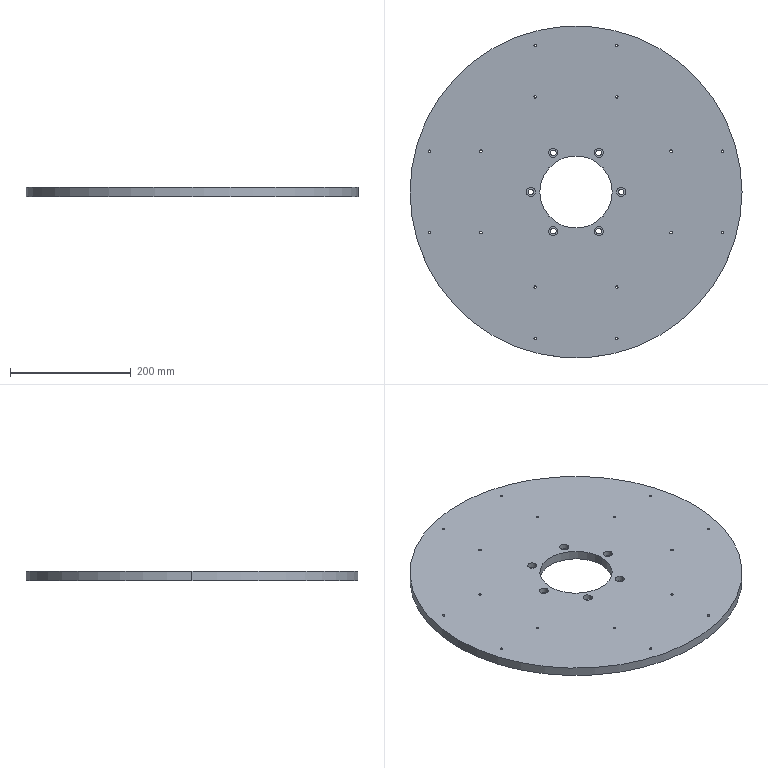Part | SolidWorks | features CirPattern 2, HoleWzd 2, Cut 1, Extrusion 1 | 1 solid | 68 faces | box 550 x 550 x 15 mm | volume 3378940 mm3 | cylinder 60 | plane 8 | commonest cylinder face diameters 4.2 x32 9 x12 15 x12 120 x2 550 x2